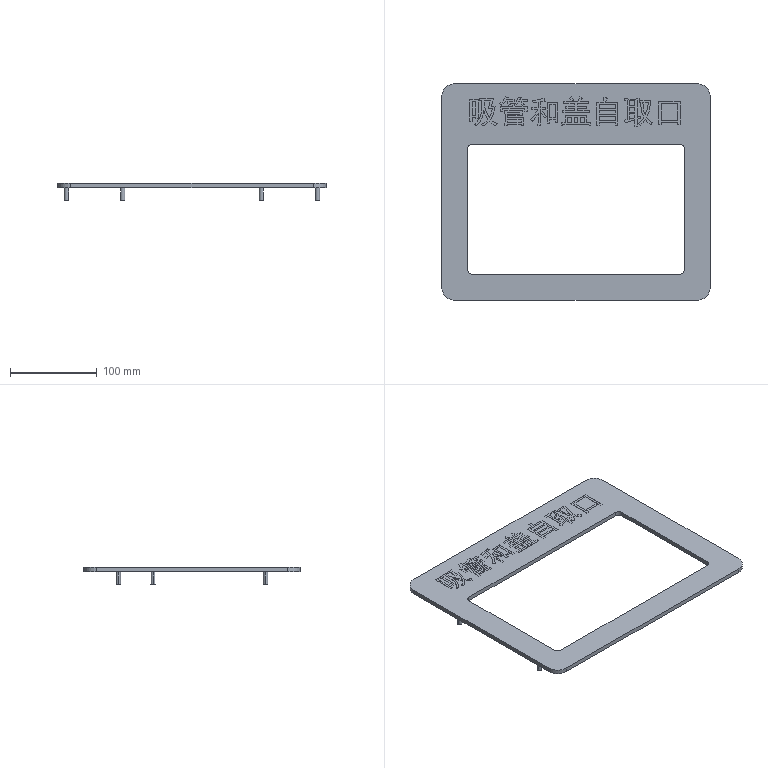Part | STEP file | Straw and lid self-pickup opening 001 | 23 solids | 387 faces | box 310 x 250 x 20.1 mm | volume 200534 mm3 | plane 225 | spline 130 | cylinder 32 | commonest cylinder face diameters 3 x12 5 x12 10 x4 30 x4